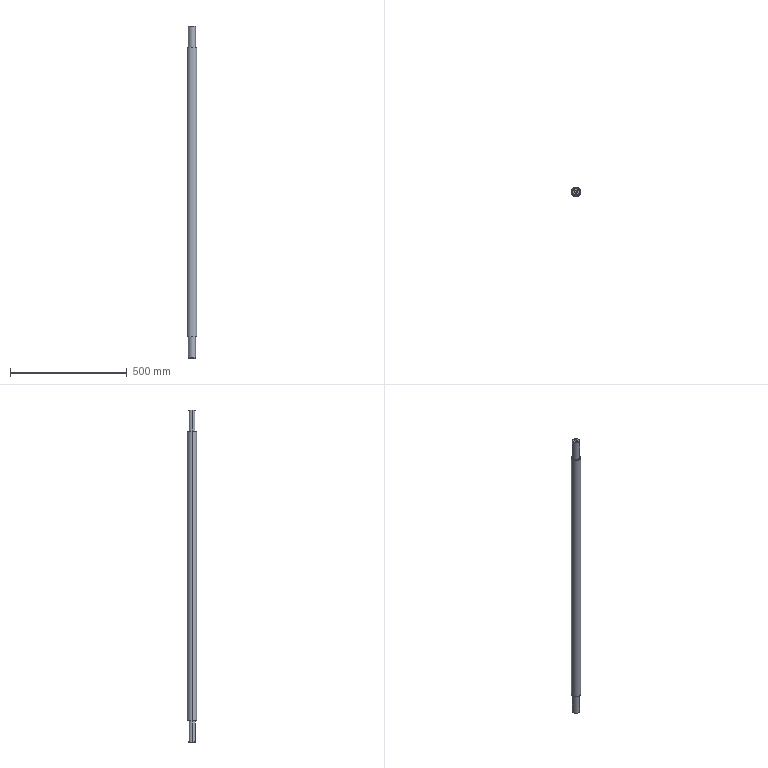Part | SolidWorks | features HoleWzd 2, Chamfer 1, Extrusion 1, ICE 1 | 1 solid | 26 faces | box 40 x 40 x 1420 mm | volume 1677021 mm3 | cone 12 | cylinder 10 | plane 4 | commonest cylinder face diameters 12 x4 30 x4 40 x2
STEP:
#1=CARTESIAN_POINT('',(-13.5,0.,-710.));
#2=VERTEX_POINT('',#1);
#3=CARTESIAN_POINT('',(13.5,0.,-710.));
#4=VERTEX_POINT('',#3);
#5=CARTESIAN_POINT('',(0.,0.,-710.));
#6=DIRECTION('',(0.,0.,-1.));
#7=DIRECTION('',(1.,0.,0.));
#8=AXIS2_PLACEMENT_3D('',#5,#6,#7);
#9=CIRCLE('',#8,13.5);
#10=EDGE_CURVE('',#2,#4,#9,.T.);
#11=ORIENTED_EDGE('',*,*,#10,.F.);
#12=CARTESIAN_POINT('',(-15.,0.,-708.5));
#13=VERTEX_POINT('',#12);
#14=CARTESIAN_POINT('',(-15.,0.,-708.5));
#15=DIRECTION('',(-0.7071,0.,0.7071));
#16=VECTOR('',#15,1000.);
#17=LINE('',#14,#16);
#18=EDGE_CURVE('',#2,#13,#17,.T.);
#19=ORIENTED_EDGE('',*,*,#18,.T.);
#20=CARTESIAN_POINT('',(15.,0.,-708.5));
#21=VERTEX_POINT('',#20);
#22=CARTESIAN_POINT('',(0.,0.,-708.5));
#23=DIRECTION('',(0.,0.,1.));
#24=DIRECTION('',(1.,0.,0.));
#25=AXIS2_PLACEMENT_3D('',#22,#23,#24);
#26=CIRCLE('',#25,15.);
#27=EDGE_CURVE('',#21,#13,#26,.T.);
#28=ORIENTED_EDGE('',*,*,#27,.F.);
#29=CARTESIAN_POINT('',(15.,0.,-708.5));
#30=DIRECTION('',(0.7071,0.,0.7071));
#31=VECTOR('',#30,1000.);
#32=LINE('',#29,#31);
#33=EDGE_CURVE('',#4,#21,#32,.T.);
#34=ORIENTED_EDGE('',*,*,#33,.F.);
#35=EDGE_LOOP('',(#11,#19,#28,#34));
#36=FACE_OUTER_BOUND('',#35,.T.);
#37=CARTESIAN_POINT('',(0.,0.,-708.5));
#38=DIRECTION('',(0.,0.,1.));
#39=DIRECTION('',(1.,0.,0.));
#40=AXIS2_PLACEMENT_3D('',#37,#38,#39);
#41=CONICAL_SURFACE('',#40,15.,0.7854);
#42=ADVANCED_FACE('',(#36),#41,.T.);
#43=CARTESIAN_POINT('',(-18.5,0.,-620.));
#44=VERTEX_POINT('',#43);
#45=CARTESIAN_POINT('',(18.5,0.,-620.));
#46=VERTEX_POINT('',#45);
#47=CARTESIAN_POINT('',(0.,0.,-620.));
#48=DIRECTION('',(0.,0.,-1.));
#49=DIRECTION('',(1.,0.,0.));
#50=AXIS2_PLACEMENT_3D('',#47,#48,#49);
#51=CIRCLE('',#50,18.5);
#52=EDGE_CURVE('',#44,#46,#51,.T.);
#53=ORIENTED_EDGE('',*,*,#52,.F.);
#54=CARTESIAN_POINT('',(-20.,0.,-618.5));
#55=VERTEX_POINT('',#54);
#56=CARTESIAN_POINT('',(-20.,0.,-618.5));
#57=DIRECTION('',(-0.7071,0.,0.7071));
#58=VECTOR('',#57,1000.);
#59=LINE('',#56,#58);
#60=EDGE_CURVE('',#44,#55,#59,.T.);
#61=ORIENTED_EDGE('',*,*,#60,.T.);
#62=CARTESIAN_POINT('',(20.,0.,-618.5));
#63=VERTEX_POINT('',#62);
#64=CARTESIAN_POINT('',(0.,0.,-618.5));
#65=DIRECTION('',(0.,0.,1.));
#66=DIRECTION('',(1.,0.,0.));
#67=AXIS2_PLACEMENT_3D('',#64,#65,#66);
#68=CIRCLE('',#67,20.);
#69=EDGE_CURVE('',#63,#55,#68,.T.);
#70=ORIENTED_EDGE('',*,*,#69,.F.);
#71=CARTESIAN_POINT('',(20.,0.,-618.5));
#72=DIRECTION('',(0.7071,0.,0.7071));
#73=VECTOR('',#72,1000.);
#74=LINE('',#71,#73);
#75=EDGE_CURVE('',#46,#63,#74,.T.);
#76=ORIENTED_EDGE('',*,*,#75,.F.);
#77=EDGE_LOOP('',(#53,#61,#70,#76));
#78=FACE_OUTER_BOUND('',#77,.T.);
#79=CARTESIAN_POINT('',(0.,0.,-618.5));
#80=DIRECTION('',(0.,0.,1.));
#81=DIRECTION('',(1.,0.,0.));
#82=AXIS2_PLACEMENT_3D('',#79,#80,#81);
#83=CONICAL_SURFACE('',#82,20.,0.7854);
#84=ADVANCED_FACE('',(#78),#83,.T.);
#85=CARTESIAN_POINT('',(18.5,0.,620.));
#86=VERTEX_POINT('',#85);
#87=CARTESIAN_POINT('',(-18.5,0.,620.));
#88=VERTEX_POINT('',#87);
#89=CARTESIAN_POINT('',(0.,0.,620.));
#90=DIRECTION('',(0.,0.,1.));
#91=DIRECTION('',(1.,0.,0.));
#92=AXIS2_PLACEMENT_3D('',#89,#90,#91);
#93=CIRCLE('',#92,18.5);
#94=EDGE_CURVE('',#86,#88,#93,.T.);
#95=ORIENTED_EDGE('',*,*,#94,.F.);
#96=CARTESIAN_POINT('',(20.,0.,618.5));
#97=VERTEX_POINT('',#96);
#98=CARTESIAN_POINT('',(18.5,0.,620.));
#99=DIRECTION('',(0.7071,0.,-0.7071));
#100=VECTOR('',#99,1000.);
#101=LINE('',#98,#100);
#102=EDGE_CURVE('',#86,#97,#101,.T.);
#103=ORIENTED_EDGE('',*,*,#102,.T.);
#104=CARTESIAN_POINT('',(-20.,0.,618.5));
#105=VERTEX_POINT('',#104);
#106=CARTESIAN_POINT('',(0.,0.,618.5));
#107=DIRECTION('',(0.,0.,-1.));
#108=DIRECTION('',(1.,0.,0.));
#109=AXIS2_PLACEMENT_3D('',#106,#107,#108);
#110=CIRCLE('',#109,20.);
#111=EDGE_CURVE('',#105,#97,#110,.T.);
#112=ORIENTED_EDGE('',*,*,#111,.F.);
#113=CARTESIAN_POINT('',(-18.5,0.,620.));
#114=DIRECTION('',(-0.7071,0.,-0.7071));
#115=VECTOR('',#114,1000.);
#116=LINE('',#113,#115);
#117=EDGE_CURVE('',#88,#105,#116,.T.);
#118=ORIENTED_EDGE('',*,*,#117,.F.);
#119=EDGE_LOOP('',(#95,#103,#112,#118));
#120=FACE_OUTER_BOUND('',#119,.T.);
#121=CARTESIAN_POINT('',(0.,0.,620.));
#122=DIRECTION('',(0.,0.,-1.));
#123=DIRECTION('',(-1.,0.,0.));
#124=AXIS2_PLACEMENT_3D('',#121,#122,#123);
#125=CONICAL_SURFACE('',#124,18.5,0.7854);
#126=ADVANCED_FACE('',(#120),#125,.T.);
#127=CARTESIAN_POINT('',(13.5,0.,710.));
#128=VERTEX_POINT('',#127);
#129=CARTESIAN_POINT('',(-13.5,0.,710.));
#130=VERTEX_POINT('',#129);
#131=CARTESIAN_POINT('',(0.,0.,710.));
#132=DIRECTION('',(0.,0.,1.));
#133=DIRECTION('',(1.,0.,0.));
#134=AXIS2_PLACEMENT_3D('',#131,#132,#133);
#135=CIRCLE('',#134,13.5);
#136=EDGE_CURVE('',#128,#130,#135,.T.);
#137=ORIENTED_EDGE('',*,*,#136,.F.);
#138=CARTESIAN_POINT('',(15.,0.,708.5));
#139=VERTEX_POINT('',#138);
#140=CARTESIAN_POINT('',(13.5,0.,710.));
#141=DIRECTION('',(0.7071,0.,-0.7071));
#142=VECTOR('',#141,1000.);
#143=LINE('',#140,#142);
#144=EDGE_CURVE('',#128,#139,#143,.T.);
#145=ORIENTED_EDGE('',*,*,#144,.T.);
#146=CARTESIAN_POINT('',(-15.,0.,708.5));
#147=VERTEX_POINT('',#146);
#148=CARTESIAN_POINT('',(0.,0.,708.5));
#149=DIRECTION('',(0.,0.,-1.));
#150=DIRECTION('',(1.,0.,0.));
#151=AXIS2_PLACEMENT_3D('',#148,#149,#150);
#152=CIRCLE('',#151,15.);
#153=EDGE_CURVE('',#147,#139,#152,.T.);
#154=ORIENTED_EDGE('',*,*,#153,.F.);
#155=CARTESIAN_POINT('',(-13.5,0.,710.));
#156=DIRECTION('',(-0.7071,0.,-0.7071));
#157=VECTOR('',#156,1000.);
#158=LINE('',#155,#157);
#159=EDGE_CURVE('',#130,#147,#158,.T.);
#160=ORIENTED_EDGE('',*,*,#159,.F.);
#161=EDGE_LOOP('',(#137,#145,#154,#160));
#162=FACE_OUTER_BOUND('',#161,.T.);
#163=CARTESIAN_POINT('',(0.,0.,710.));
#164=DIRECTION('',(0.,0.,-1.));
#165=DIRECTION('',(-1.,0.,0.));
#166=AXIS2_PLACEMENT_3D('',#163,#164,#165);
#167=CONICAL_SURFACE('',#166,13.5,0.7854);
#168=ADVANCED_FACE('',(#162),#167,.T.);
#169=CARTESIAN_POINT('',(15.,0.,-620.));
#170=VERTEX_POINT('',#169);
#171=CARTESIAN_POINT('',(-15.,0.,-620.));
#172=VERTEX_POINT('',#171);
#173=CARTESIAN_POINT('',(0.,0.,-620.));
#174=DIRECTION('',(0.,0.,1.));
#175=DIRECTION('',(1.,0.,0.));
#176=AXIS2_PLACEMENT_3D('',#173,#174,#175);
#177=CIRCLE('',#176,15.);
#178=EDGE_CURVE('',#170,#172,#177,.T.);
#179=ORIENTED_EDGE('',*,*,#178,.F.);
#180=CARTESIAN_POINT('',(15.,0.,710.));
#181=DIRECTION('',(0.,0.,-1.));
#182=VECTOR('',#181,1000.);
#183=LINE('',#180,#182);
#184=EDGE_CURVE('',#170,#21,#183,.T.);
#185=ORIENTED_EDGE('',*,*,#184,.T.);
#186=ORIENTED_EDGE('',*,*,#27,.T.);
#187=CARTESIAN_POINT('',(-15.,0.,710.));
#188=DIRECTION('',(0.,0.,-1.));
#189=VECTOR('',#188,1000.);
#190=LINE('',#187,#189);
#191=EDGE_CURVE('',#172,#13,#190,.T.);
#192=ORIENTED_EDGE('',*,*,#191,.F.);
#193=EDGE_LOOP('',(#179,#185,#186,#192));
#194=FACE_OUTER_BOUND('',#193,.T.);
#195=CARTESIAN_POINT('',(0.,0.,710.));
#196=DIRECTION('',(0.,0.,-1.));
#197=DIRECTION('',(-1.,0.,0.));
#198=AXIS2_PLACEMENT_3D('',#195,#196,#197);
#199=CYLINDRICAL_SURFACE('',#198,15.);
#200=ADVANCED_FACE('',(#194),#199,.T.);
#201=CARTESIAN_POINT('',(6.,0.,-676.));
#202=VERTEX_POINT('',#201);
#203=CARTESIAN_POINT('',(-6.,0.,-676.));
#204=VERTEX_POINT('',#203);
#205=CARTESIAN_POINT('',(0.,0.,-676.));
#206=DIRECTION('',(0.,0.,-1.));
#207=DIRECTION('',(-1.,0.,0.));
#208=AXIS2_PLACEMENT_3D('',#205,#206,#207);
#209=CIRCLE('',#208,6.);
#210=EDGE_CURVE('',#202,#204,#209,.T.);
#211=ORIENTED_EDGE('',*,*,#210,.F.);
#212=CARTESIAN_POINT('',(6.,0.,-710.));
#213=VERTEX_POINT('',#212);
#214=CARTESIAN_POINT('',(6.,0.,-710.));
#215=DIRECTION('',(0.,0.,-1.));
#216=VECTOR('',#215,1000.);
#217=LINE('',#214,#216);
#218=EDGE_CURVE('',#202,#213,#217,.T.);
#219=ORIENTED_EDGE('',*,*,#218,.T.);
#220=CARTESIAN_POINT('',(-6.,0.,-710.));
#221=VERTEX_POINT('',#220);
#222=CARTESIAN_POINT('',(0.,0.,-710.));
#223=DIRECTION('',(0.,0.,-1.));
#224=DIRECTION('',(-1.,0.,0.));
#225=AXIS2_PLACEMENT_3D('',#222,#223,#224);
#226=CIRCLE('',#225,6.);
#227=EDGE_CURVE('',#213,#221,#226,.T.);
#228=ORIENTED_EDGE('',*,*,#227,.T.);
#229=CARTESIAN_POINT('',(-6.,0.,-710.));
#230=DIRECTION('',(0.,0.,-1.));
#231=VECTOR('',#230,1000.);
#232=LINE('',#229,#231);
#233=EDGE_CURVE('',#204,#221,#232,.T.);
#234=ORIENTED_EDGE('',*,*,#233,.F.);
#235=EDGE_LOOP('',(#211,#219,#228,#234));
#236=FACE_OUTER_BOUND('',#235,.T.);
#237=CARTESIAN_POINT('',(0.,0.,-710.));
#238=DIRECTION('',(0.,0.,-1.));
#239=DIRECTION('',(-1.,0.,0.));
#240=AXIS2_PLACEMENT_3D('',#237,#238,#239);
#241=CYLINDRICAL_SURFACE('',#240,6.);
#242=ADVANCED_FACE('',(#236),#241,.F.);
#243=CARTESIAN_POINT('',(0.,0.,-672.395));
#244=VERTEX_POINT('',#243);
#245=CARTESIAN_POINT('',(-6.,0.,-676.));
#246=DIRECTION('',(-0.8572,0.,-0.515));
#247=VECTOR('',#246,1000.);
#248=LINE('',#245,#247);
#249=EDGE_CURVE('',#244,#204,#248,.T.);
#250=ORIENTED_EDGE('',*,*,#249,.F.);
#251=CARTESIAN_POINT('',(6.,0.,-676.));
#252=DIRECTION('',(0.8572,0.,-0.515));
#253=VECTOR('',#252,1000.);
#254=LINE('',#251,#253);
#255=EDGE_CURVE('',#244,#202,#254,.T.);
#256=ORIENTED_EDGE('',*,*,#255,.T.);
#257=ORIENTED_EDGE('',*,*,#210,.T.);
#258=EDGE_LOOP('',(#250,#256,#257));
#259=FACE_OUTER_BOUND('',#258,.T.);
#260=CARTESIAN_POINT('',(0.,0.,-676.));
#261=DIRECTION('',(0.,0.,-1.));
#262=DIRECTION('',(-1.,0.,0.));
#263=AXIS2_PLACEMENT_3D('',#260,#261,#262);
#264=CONICAL_SURFACE('',#263,6.,1.03);
#265=ADVANCED_FACE('',(#259),#264,.F.);
#266=ORIENTED_EDGE('',*,*,#111,.T.);
#267=CARTESIAN_POINT('',(20.,0.,620.));
#268=DIRECTION('',(0.,0.,-1.));
#269=VECTOR('',#268,1000.);
#270=LINE('',#267,#269);
#271=EDGE_CURVE('',#97,#63,#270,.T.);
#272=ORIENTED_EDGE('',*,*,#271,.T.);
#273=ORIENTED_EDGE('',*,*,#69,.T.);
#274=CARTESIAN_POINT('',(-20.,0.,620.));
#275=DIRECTION('',(0.,0.,-1.));
#276=VECTOR('',#275,1000.);
#277=LINE('',#274,#276);
#278=EDGE_CURVE('',#105,#55,#277,.T.);
#279=ORIENTED_EDGE('',*,*,#278,.F.);
#280=EDGE_LOOP('',(#266,#272,#273,#279));
#281=FACE_OUTER_BOUND('',#280,.T.);
#282=CARTESIAN_POINT('',(0.,0.,620.));
#283=DIRECTION('',(0.,0.,-1.));
#284=DIRECTION('',(-1.,0.,0.));
#285=AXIS2_PLACEMENT_3D('',#282,#283,#284);
#286=CYLINDRICAL_SURFACE('',#285,20.);
#287=ADVANCED_FACE('',(#281),#286,.T.);
#288=CARTESIAN_POINT('',(-6.,0.,676.));
#289=VERTEX_POINT('',#288);
#290=CARTESIAN_POINT('',(6.,0.,676.));
#291=VERTEX_POINT('',#290);
#292=CARTESIAN_POINT('',(0.,0.,676.));
#293=DIRECTION('',(0.,0.,1.));
#294=DIRECTION('',(1.,0.,0.));
#295=AXIS2_PLACEMENT_3D('',#292,#293,#294);
#296=CIRCLE('',#295,6.);
#297=EDGE_CURVE('',#289,#291,#296,.T.);
#298=ORIENTED_EDGE('',*,*,#297,.F.);
#299=CARTESIAN_POINT('',(-6.,0.,710.));
#300=VERTEX_POINT('',#299);
#301=CARTESIAN_POINT('',(-6.,0.,710.));
#302=DIRECTION('',(0.,0.,1.));
#303=VECTOR('',#302,1000.);
#304=LINE('',#301,#303);
#305=EDGE_CURVE('',#289,#300,#304,.T.);
#306=ORIENTED_EDGE('',*,*,#305,.T.);
#307=CARTESIAN_POINT('',(6.,0.,710.));
#308=VERTEX_POINT('',#307);
#309=CARTESIAN_POINT('',(0.,0.,710.));
#310=DIRECTION('',(0.,0.,1.));
#311=DIRECTION('',(1.,0.,0.));
#312=AXIS2_PLACEMENT_3D('',#309,#310,#311);
#313=CIRCLE('',#312,6.);
#314=EDGE_CURVE('',#300,#308,#313,.T.);
#315=ORIENTED_EDGE('',*,*,#314,.T.);
#316=CARTESIAN_POINT('',(6.,0.,710.));
#317=DIRECTION('',(0.,0.,1.));
#318=VECTOR('',#317,1000.);
#319=LINE('',#316,#318);
#320=EDGE_CURVE('',#291,#308,#319,.T.);
#321=ORIENTED_EDGE('',*,*,#320,.F.);
#322=EDGE_LOOP('',(#298,#306,#315,#321));
#323=FACE_OUTER_BOUND('',#322,.T.);
#324=CARTESIAN_POINT('',(0.,0.,710.));
#325=DIRECTION('',(0.,0.,1.));
#326=DIRECTION('',(1.,0.,0.));
#327=AXIS2_PLACEMENT_3D('',#324,#325,#326);
#328=CYLINDRICAL_SURFACE('',#327,6.);
#329=ADVANCED_FACE('',(#323),#328,.F.);
#330=CARTESIAN_POINT('',(0.,0.,672.395));
#331=VERTEX_POINT('',#330);
#332=CARTESIAN_POINT('',(6.,0.,676.));
#333=DIRECTION('',(0.8572,0.,0.515));
#334=VECTOR('',#333,1000.);
#335=LINE('',#332,#334);
#336=EDGE_CURVE('',#331,#291,#335,.T.);
#337=ORIENTED_EDGE('',*,*,#336,.F.);
#338=CARTESIAN_POINT('',(-6.,0.,676.));
#339=DIRECTION('',(-0.8572,0.,0.515));
#340=VECTOR('',#339,1000.);
#341=LINE('',#338,#340);
#342=EDGE_CURVE('',#331,#289,#341,.T.);
#343=ORIENTED_EDGE('',*,*,#342,.T.);
#344=ORIENTED_EDGE('',*,*,#297,.T.);
#345=EDGE_LOOP('',(#337,#343,#344));
#346=FACE_OUTER_BOUND('',#345,.T.);
#347=CARTESIAN_POINT('',(0.,0.,676.));
#348=DIRECTION('',(0.,0.,1.));
#349=DIRECTION('',(1.,0.,0.));
#350=AXIS2_PLACEMENT_3D('',#347,#348,#349);
#351=CONICAL_SURFACE('',#350,6.,1.03);
#352=ADVANCED_FACE('',(#346),#351,.F.);
#353=ORIENTED_EDGE('',*,*,#153,.T.);
#354=CARTESIAN_POINT('',(15.,0.,620.));
#355=VERTEX_POINT('',#354);
#356=CARTESIAN_POINT('',(15.,0.,710.));
#357=DIRECTION('',(0.,0.,-1.));
#358=VECTOR('',#357,1000.);
#359=LINE('',#356,#358);
#360=EDGE_CURVE('',#139,#355,#359,.T.);
#361=ORIENTED_EDGE('',*,*,#360,.T.);
#362=CARTESIAN_POINT('',(-15.,0.,620.));
#363=VERTEX_POINT('',#362);
#364=CARTESIAN_POINT('',(0.,0.,620.));
#365=DIRECTION('',(0.,0.,1.));
#366=DIRECTION('',(1.,0.,0.));
#367=AXIS2_PLACEMENT_3D('',#364,#365,#366);
#368=CIRCLE('',#367,15.);
#369=EDGE_CURVE('',#355,#363,#368,.T.);
#370=ORIENTED_EDGE('',*,*,#369,.T.);
#371=CARTESIAN_POINT('',(-15.,0.,710.));
#372=DIRECTION('',(0.,0.,-1.));
#373=VECTOR('',#372,1000.);
#374=LINE('',#371,#373);
#375=EDGE_CURVE('',#147,#363,#374,.T.);
#376=ORIENTED_EDGE('',*,*,#375,.F.);
#377=EDGE_LOOP('',(#353,#361,#370,#376));
#378=FACE_OUTER_BOUND('',#377,.T.);
#379=CARTESIAN_POINT('',(0.,0.,710.));
#380=DIRECTION('',(0.,0.,-1.));
#381=DIRECTION('',(-1.,0.,0.));
#382=AXIS2_PLACEMENT_3D('',#379,#380,#381);
#383=CYLINDRICAL_SURFACE('',#382,15.);
#384=ADVANCED_FACE('',(#378),#383,.T.);
#385=ORIENTED_EDGE('',*,*,#360,.F.);
#386=CARTESIAN_POINT('',(0.,0.,708.5));
#387=DIRECTION('',(0.,0.,-1.));
#388=DIRECTION('',(1.,0.,0.));
#389=AXIS2_PLACEMENT_3D('',#386,#387,#388);
#390=CIRCLE('',#389,15.);
#391=EDGE_CURVE('',#139,#147,#390,.T.);
#392=ORIENTED_EDGE('',*,*,#391,.T.);
#393=ORIENTED_EDGE('',*,*,#375,.T.);
#394=CARTESIAN_POINT('',(0.,0.,620.));
#395=DIRECTION('',(0.,0.,1.));
#396=DIRECTION('',(1.,0.,0.));
#397=AXIS2_PLACEMENT_3D('',#394,#395,#396);
#398=CIRCLE('',#397,15.);
#399=EDGE_CURVE('',#363,#355,#398,.T.);
#400=ORIENTED_EDGE('',*,*,#399,.T.);
#401=EDGE_LOOP('',(#385,#392,#393,#400));
#402=FACE_OUTER_BOUND('',#401,.T.);
#403=CARTESIAN_POINT('',(0.,0.,710.));
#404=DIRECTION('',(0.,0.,-1.));
#405=DIRECTION('',(-1.,0.,0.));
#406=AXIS2_PLACEMENT_3D('',#403,#404,#405);
#407=CYLINDRICAL_SURFACE('',#406,15.);
#408=ADVANCED_FACE('',(#402),#407,.T.);
#409=CARTESIAN_POINT('',(0.,0.,710.));
#410=DIRECTION('',(0.,0.,1.));
#411=DIRECTION('',(1.,0.,0.));
#412=AXIS2_PLACEMENT_3D('',#409,#410,#411);
#413=CIRCLE('',#412,13.5);
#414=EDGE_CURVE('',#130,#128,#413,.T.);
#415=ORIENTED_EDGE('',*,*,#414,.T.);
#416=ORIENTED_EDGE('',*,*,#136,.T.);
#417=EDGE_LOOP('',(#415,#416));
#418=FACE_OUTER_BOUND('',#417,.T.);
#419=CARTESIAN_POINT('',(0.,0.,710.));
#420=DIRECTION('',(0.,0.,1.));
#421=DIRECTION('',(1.,0.,0.));
#422=AXIS2_PLACEMENT_3D('',#419,#420,#421);
#423=CIRCLE('',#422,6.);
#424=EDGE_CURVE('',#308,#300,#423,.T.);
#425=ORIENTED_EDGE('',*,*,#424,.F.);
#426=ORIENTED_EDGE('',*,*,#314,.F.);
#427=EDGE_LOOP('',(#425,#426));
#428=FACE_BOUND('',#427,.T.);
#429=CARTESIAN_POINT('',(0.,0.,710.));
#430=DIRECTION('',(0.,0.,1.));
#431=DIRECTION('',(1.,0.,0.));
#432=AXIS2_PLACEMENT_3D('',#429,#430,#431);
#433=PLANE('',#432);
#434=ADVANCED_FACE('',(#418,#428),#433,.T.);
#435=ORIENTED_EDGE('',*,*,#342,.F.);
#436=ORIENTED_EDGE('',*,*,#336,.T.);
#437=CARTESIAN_POINT('',(0.,0.,676.));
#438=DIRECTION('',(0.,0.,1.));
#439=DIRECTION('',(1.,0.,0.));
#440=AXIS2_PLACEMENT_3D('',#437,#438,#439);
#441=CIRCLE('',#440,6.);
#442=EDGE_CURVE('',#291,#289,#441,.T.);
#443=ORIENTED_EDGE('',*,*,#442,.T.);
#444=EDGE_LOOP('',(#435,#436,#443));
#445=FACE_OUTER_BOUND('',#444,.T.);
#446=CARTESIAN_POINT('',(0.,0.,676.));
#447=DIRECTION('',(0.,0.,1.));
#448=DIRECTION('',(1.,0.,0.));
#449=AXIS2_PLACEMENT_3D('',#446,#447,#448);
#450=CONICAL_SURFACE('',#449,6.,1.03);
#451=ADVANCED_FACE('',(#445),#450,.F.);
#452=ORIENTED_EDGE('',*,*,#305,.F.);
#453=ORIENTED_EDGE('',*,*,#442,.F.);
#454=ORIENTED_EDGE('',*,*,#320,.T.);
#455=ORIENTED_EDGE('',*,*,#424,.T.);
#456=EDGE_LOOP('',(#452,#453,#454,#455));
#457=FACE_OUTER_BOUND('',#456,.T.);
#458=CARTESIAN_POINT('',(0.,0.,710.));
#459=DIRECTION('',(0.,0.,1.));
#460=DIRECTION('',(1.,0.,0.));
#461=AXIS2_PLACEMENT_3D('',#458,#459,#460);
#462=CYLINDRICAL_SURFACE('',#461,6.);
#463=ADVANCED_FACE('',(#457),#462,.F.);
#464=ORIENTED_EDGE('',*,*,#271,.F.);
#465=CARTESIAN_POINT('',(0.,0.,618.5));
#466=DIRECTION('',(0.,0.,-1.));
#467=DIRECTION('',(1.,0.,0.));
#468=AXIS2_PLACEMENT_3D('',#465,#466,#467);
#469=CIRCLE('',#468,20.);
#470=EDGE_CURVE('',#97,#105,#469,.T.);
#471=ORIENTED_EDGE('',*,*,#470,.T.);
#472=ORIENTED_EDGE('',*,*,#278,.T.);
#473=CARTESIAN_POINT('',(0.,0.,-618.5));
#474=DIRECTION('',(0.,0.,1.));
#475=DIRECTION('',(1.,0.,0.));
#476=AXIS2_PLACEMENT_3D('',#473,#474,#475);
#477=CIRCLE('',#476,20.);
#478=EDGE_CURVE('',#55,#63,#477,.T.);
#479=ORIENTED_EDGE('',*,*,#478,.T.);
#480=EDGE_LOOP('',(#464,#471,#472,#479));
#481=FACE_OUTER_BOUND('',#480,.T.);
#482=CARTESIAN_POINT('',(0.,0.,620.));
#483=DIRECTION('',(0.,0.,-1.));
#484=DIRECTION('',(-1.,0.,0.));
#485=AXIS2_PLACEMENT_3D('',#482,#483,#484);
#486=CYLINDRICAL_SURFACE('',#485,20.);
#487=ADVANCED_FACE('',(#481),#486,.T.);
#488=CARTESIAN_POINT('',(0.,0.,620.));
#489=DIRECTION('',(0.,0.,1.));
#490=DIRECTION('',(1.,0.,0.));
#491=AXIS2_PLACEMENT_3D('',#488,#489,#490);
#492=CIRCLE('',#491,18.5);
#493=EDGE_CURVE('',#88,#86,#492,.T.);
#494=ORIENTED_EDGE('',*,*,#493,.T.);
#495=ORIENTED_EDGE('',*,*,#94,.T.);
#496=EDGE_LOOP('',(#494,#495));
#497=FACE_OUTER_BOUND('',#496,.T.);
#498=ORIENTED_EDGE('',*,*,#399,.F.);
#499=ORIENTED_EDGE('',*,*,#369,.F.);
#500=EDGE_LOOP('',(#498,#499));
#501=FACE_BOUND('',#500,.T.);
#502=CARTESIAN_POINT('',(0.,0.,620.));
#503=DIRECTION('',(0.,0.,1.));
#504=DIRECTION('',(1.,0.,0.));
#505=AXIS2_PLACEMENT_3D('',#502,#503,#504);
#506=PLANE('',#505);
#507=ADVANCED_FACE('',(#497,#501),#506,.T.);
#508=CARTESIAN_POINT('',(0.,0.,-620.));
#509=DIRECTION('',(0.,0.,-1.));
#510=DIRECTION('',(1.,0.,0.));
#511=AXIS2_PLACEMENT_3D('',#508,#509,#510);
#512=CIRCLE('',#511,18.5);
#513=EDGE_CURVE('',#46,#44,#512,.T.);
#514=ORIENTED_EDGE('',*,*,#513,.T.);
#515=ORIENTED_EDGE('',*,*,#52,.T.);
#516=EDGE_LOOP('',(#514,#515));
#517=FACE_OUTER_BOUND('',#516,.T.);
#518=CARTESIAN_POINT('',(0.,0.,-620.));
#519=DIRECTION('',(0.,0.,1.));
#520=DIRECTION('',(1.,0.,0.));
#521=AXIS2_PLACEMENT_3D('',#518,#519,#520);
#522=CIRCLE('',#521,15.);
#523=EDGE_CURVE('',#172,#170,#522,.T.);
#524=ORIENTED_EDGE('',*,*,#523,.T.);
#525=ORIENTED_EDGE('',*,*,#178,.T.);
#526=EDGE_LOOP('',(#524,#525));
#527=FACE_BOUND('',#526,.T.);
#528=CARTESIAN_POINT('',(0.,0.,-620.));
#529=DIRECTION('',(0.,0.,1.));
#530=DIRECTION('',(1.,0.,0.));
#531=AXIS2_PLACEMENT_3D('',#528,#529,#530);
#532=PLANE('',#531);
#533=ADVANCED_FACE('',(#517,#527),#532,.F.);
#534=ORIENTED_EDGE('',*,*,#255,.F.);
#535=ORIENTED_EDGE('',*,*,#249,.T.);
#536=CARTESIAN_POINT('',(0.,0.,-676.));
#537=DIRECTION('',(0.,0.,-1.));
#538=DIRECTION('',(-1.,0.,0.));
#539=AXIS2_PLACEMENT_3D('',#536,#537,#538);
#540=CIRCLE('',#539,6.);
#541=EDGE_CURVE('',#204,#202,#540,.T.);
#542=ORIENTED_EDGE('',*,*,#541,.T.);
#543=EDGE_LOOP('',(#534,#535,#542));
#544=FACE_OUTER_BOUND('',#543,.T.);
#545=CARTESIAN_POINT('',(0.,0.,-676.));
#546=DIRECTION('',(0.,0.,-1.));
#547=DIRECTION('',(-1.,0.,0.));
#548=AXIS2_PLACEMENT_3D('',#545,#546,#547);
#549=CONICAL_SURFACE('',#548,6.,1.03);
#550=ADVANCED_FACE('',(#544),#549,.F.);
#551=ORIENTED_EDGE('',*,*,#218,.F.);
#552=ORIENTED_EDGE('',*,*,#541,.F.);
#553=ORIENTED_EDGE('',*,*,#233,.T.);
#554=CARTESIAN_POINT('',(0.,0.,-710.));
#555=DIRECTION('',(0.,0.,-1.));
#556=DIRECTION('',(-1.,0.,0.));
#557=AXIS2_PLACEMENT_3D('',#554,#555,#556);
#558=CIRCLE('',#557,6.);
#559=EDGE_CURVE('',#221,#213,#558,.T.);
#560=ORIENTED_EDGE('',*,*,#559,.T.);
#561=EDGE_LOOP('',(#551,#552,#553,#560));
#562=FACE_OUTER_BOUND('',#561,.T.);
#563=CARTESIAN_POINT('',(0.,0.,-710.));
#564=DIRECTION('',(0.,0.,-1.));
#565=DIRECTION('',(-1.,0.,0.));
#566=AXIS2_PLACEMENT_3D('',#563,#564,#565);
#567=CYLINDRICAL_SURFACE('',#566,6.);
#568=ADVANCED_FACE('',(#562),#567,.F.);
#569=CARTESIAN_POINT('',(0.,0.,-710.));
#570=DIRECTION('',(0.,0.,-1.));
#571=DIRECTION('',(1.,0.,0.));
#572=AXIS2_PLACEMENT_3D('',#569,#570,#571);
#573=CIRCLE('',#572,13.5);
#574=EDGE_CURVE('',#4,#2,#573,.T.);
#575=ORIENTED_EDGE('',*,*,#574,.T.);
#576=ORIENTED_EDGE('',*,*,#10,.T.);
#577=EDGE_LOOP('',(#575,#576));
#578=FACE_OUTER_BOUND('',#577,.T.);
#579=ORIENTED_EDGE('',*,*,#559,.F.);
#580=ORIENTED_EDGE('',*,*,#227,.F.);
#581=EDGE_LOOP('',(#579,#580));
#582=FACE_BOUND('',#581,.T.);
#583=CARTESIAN_POINT('',(0.,0.,-710.));
#584=DIRECTION('',(0.,0.,1.));
#585=DIRECTION('',(1.,0.,0.));
#586=AXIS2_PLACEMENT_3D('',#583,#584,#585);
#587=PLANE('',#586);
#588=ADVANCED_FACE('',(#578,#582),#587,.F.);
#589=ORIENTED_EDGE('',*,*,#184,.F.);
#590=ORIENTED_EDGE('',*,*,#523,.F.);
#591=ORIENTED_EDGE('',*,*,#191,.T.);
#592=CARTESIAN_POINT('',(0.,0.,-708.5));
#593=DIRECTION('',(0.,0.,1.));
#594=DIRECTION('',(1.,0.,0.));
#595=AXIS2_PLACEMENT_3D('',#592,#593,#594);
#596=CIRCLE('',#595,15.);
#597=EDGE_CURVE('',#13,#21,#596,.T.);
#598=ORIENTED_EDGE('',*,*,#597,.T.);
#599=EDGE_LOOP('',(#589,#590,#591,#598));
#600=FACE_OUTER_BOUND('',#599,.T.);
#601=CARTESIAN_POINT('',(0.,0.,710.));
#602=DIRECTION('',(0.,0.,-1.));
#603=DIRECTION('',(-1.,0.,0.));
#604=AXIS2_PLACEMENT_3D('',#601,#602,#603);
#605=CYLINDRICAL_SURFACE('',#604,15.);
#606=ADVANCED_FACE('',(#600),#605,.T.);
#607=ORIENTED_EDGE('',*,*,#144,.F.);
#608=ORIENTED_EDGE('',*,*,#414,.F.);
#609=ORIENTED_EDGE('',*,*,#159,.T.);
#610=ORIENTED_EDGE('',*,*,#391,.F.);
#611=EDGE_LOOP('',(#607,#608,#609,#610));
#612=FACE_OUTER_BOUND('',#611,.T.);
#613=CARTESIAN_POINT('',(0.,0.,710.));
#614=DIRECTION('',(0.,0.,-1.));
#615=DIRECTION('',(-1.,0.,0.));
#616=AXIS2_PLACEMENT_3D('',#613,#614,#615);
#617=CONICAL_SURFACE('',#616,13.5,0.7854);
#618=ADVANCED_FACE('',(#612),#617,.T.);
#619=ORIENTED_EDGE('',*,*,#102,.F.);
#620=ORIENTED_EDGE('',*,*,#493,.F.);
#621=ORIENTED_EDGE('',*,*,#117,.T.);
#622=ORIENTED_EDGE('',*,*,#470,.F.);
#623=EDGE_LOOP('',(#619,#620,#621,#622));
#624=FACE_OUTER_BOUND('',#623,.T.);
#625=CARTESIAN_POINT('',(0.,0.,620.));
#626=DIRECTION('',(0.,0.,-1.));
#627=DIRECTION('',(-1.,0.,0.));
#628=AXIS2_PLACEMENT_3D('',#625,#626,#627);
#629=CONICAL_SURFACE('',#628,18.5,0.7854);
#630=ADVANCED_FACE('',(#624),#629,.T.);
#631=ORIENTED_EDGE('',*,*,#60,.F.);
#632=ORIENTED_EDGE('',*,*,#513,.F.);
#633=ORIENTED_EDGE('',*,*,#75,.T.);
#634=ORIENTED_EDGE('',*,*,#478,.F.);
#635=EDGE_LOOP('',(#631,#632,#633,#634));
#636=FACE_OUTER_BOUND('',#635,.T.);
#637=CARTESIAN_POINT('',(0.,0.,-618.5));
#638=DIRECTION('',(0.,0.,1.));
#639=DIRECTION('',(1.,0.,0.));
#640=AXIS2_PLACEMENT_3D('',#637,#638,#639);
#641=CONICAL_SURFACE('',#640,20.,0.7854);
#642=ADVANCED_FACE('',(#636),#641,.T.);
#643=ORIENTED_EDGE('',*,*,#18,.F.);
#644=ORIENTED_EDGE('',*,*,#574,.F.);
#645=ORIENTED_EDGE('',*,*,#33,.T.);
#646=ORIENTED_EDGE('',*,*,#597,.F.);
#647=EDGE_LOOP('',(#643,#644,#645,#646));
#648=FACE_OUTER_BOUND('',#647,.T.);
#649=CARTESIAN_POINT('',(0.,0.,-708.5));
#650=DIRECTION('',(0.,0.,1.));
#651=DIRECTION('',(1.,0.,0.));
#652=AXIS2_PLACEMENT_3D('',#649,#650,#651);
#653=CONICAL_SURFACE('',#652,15.,0.7854);
#654=ADVANCED_FACE('',(#648),#653,.T.);
#655=CLOSED_SHELL('',(#42,#84,#126,#168,#200,#242,#265,#287,#329,#352,#384,#408,#434,#451,#463,#487,#507,#533,#550,#568,#588,#606,#618,#630,#642,#654));
#656=MANIFOLD_SOLID_BREP('',#655);
#657=CARTESIAN_POINT('',(0.,0.,0.));
#658=DIRECTION('',(0.,0.,1.));
#659=DIRECTION('',(1.,0.,0.));
#660=AXIS2_PLACEMENT_3D('',#657,#658,#659);
#661=(LENGTH_UNIT()NAMED_UNIT(*)SI_UNIT(.MILLI.,.METRE.));
#662=UNCERTAINTY_MEASURE_WITH_UNIT(LENGTH_MEASURE(0.00001),#661,'','');
#663=(NAMED_UNIT(*)PLANE_ANGLE_UNIT()SI_UNIT($,.RADIAN.));
#664=(NAMED_UNIT(*)SI_UNIT($,.STERADIAN.)SOLID_ANGLE_UNIT());
#665=(GEOMETRIC_REPRESENTATION_CONTEXT(3)GLOBAL_UNCERTAINTY_ASSIGNED_CONTEXT((#662))GLOBAL_UNIT_ASSIGNED_CONTEXT((#661,#663,#664))REPRESENTATION_CONTEXT('',''));
#666=ADVANCED_BREP_SHAPE_REPRESENTATION('',(#656,#660),#665);